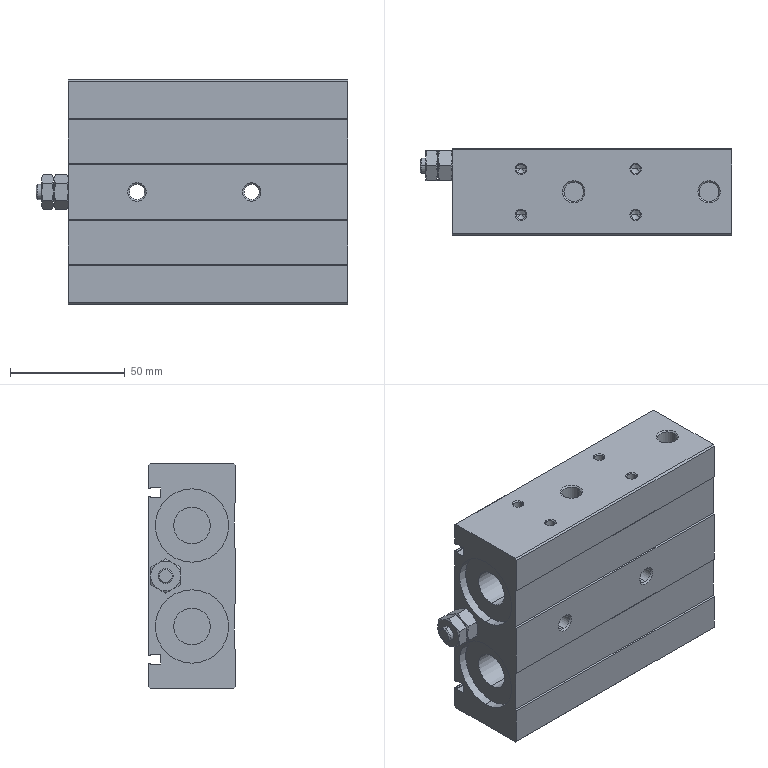Part | SolidWorks | features BaseBody 1 | 1 solid | 208 faces | box 136 x 38 x 98 mm | volume 311223 mm3 | cone 74 | cylinder 72 | plane 62 | commonest cylinder face diameters 4.134 x16 0.8 x12 8.566 x8 32 x8 0.4 x4 6.647 x4